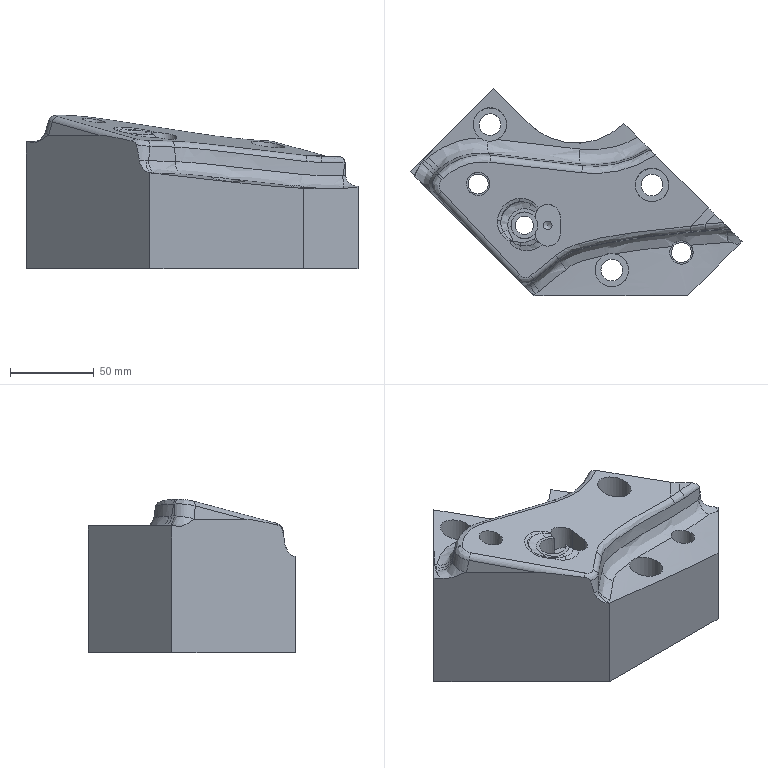Part | STEP file | gslz 2016.10.28-13_id1514_x_t | 1 solid | 98 faces | box 198.697 x 124.174 x 92.051 mm | volume 929934 mm3 | spline 50 | plane 24 | cylinder 23 | cone 1 | commonest cylinder face diameters 7.5 x4 13 x3 20 x3 12 x2 14 x2 15 x2